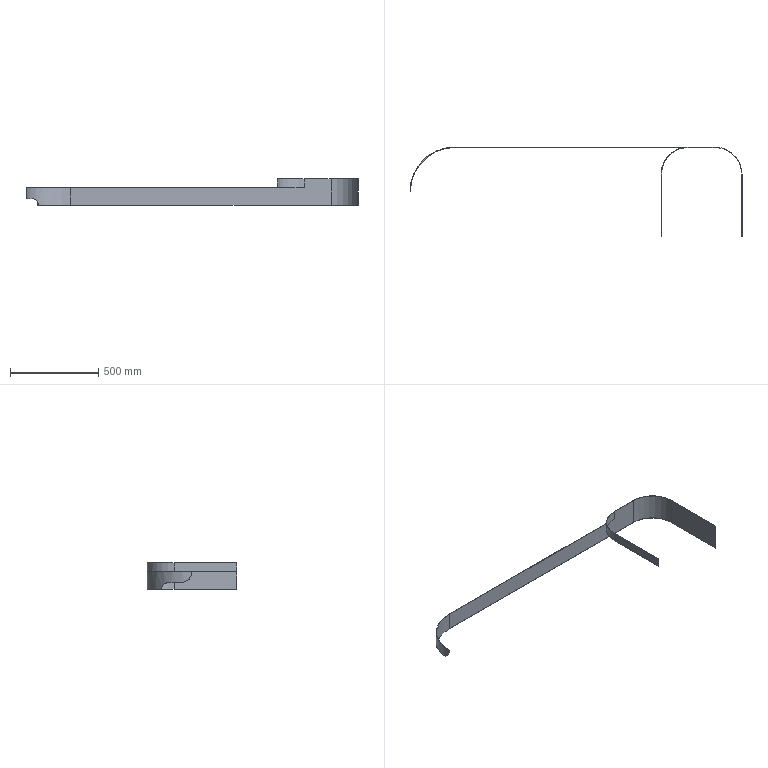Part | SolidWorks | features ICE 2, Extrusion 1 | 1 solid | 21 faces | box 1880 x 508 x 152.4 mm | volume 621350 mm3 | plane 13 | cylinder 8 | commonest cylinder face diameters 300.8 x2 304.8 x2 76.2 x1 127 x1 504 x1 508 x1
STEP:
#1=CARTESIAN_POINT('',(-215.391,134.62,-63.5));
#2=VERTEX_POINT('',#1);
#3=CARTESIAN_POINT('',(-186.236,172.72,-101.6));
#4=VERTEX_POINT('',#3);
#5=CARTESIAN_POINT('',(-215.391,134.62,-63.5));
#6=CARTESIAN_POINT('',(-213.888,137.025,-63.5));
#7=CARTESIAN_POINT('',(-212.368,139.368,-63.725));
#8=CARTESIAN_POINT('',(-209.293,143.945,-64.585));
#9=CARTESIAN_POINT('',(-207.739,146.177,-65.22));
#10=CARTESIAN_POINT('',(-205.78,148.9,-66.272));
#11=CARTESIAN_POINT('',(-205.387,149.441,-66.496));
#12=CARTESIAN_POINT('',(-204.6,150.517,-66.97));
#13=CARTESIAN_POINT('',(-204.206,151.05,-67.22));
#14=CARTESIAN_POINT('',(-203.034,152.627,-68.004));
#15=CARTESIAN_POINT('',(-202.26,153.651,-68.573));
#16=CARTESIAN_POINT('',(-199.965,156.64,-70.42));
#17=CARTESIAN_POINT('',(-198.471,158.526,-71.836));
#18=CARTESIAN_POINT('',(-196.304,161.19,-74.267));
#19=CARTESIAN_POINT('',(-195.593,162.051,-75.129));
#20=CARTESIAN_POINT('',(-194.206,163.711,-76.966));
#21=CARTESIAN_POINT('',(-193.538,164.499,-77.927));
#22=CARTESIAN_POINT('',(-192.262,165.989,-79.939));
#23=CARTESIAN_POINT('',(-191.654,166.69,-80.991));
#24=CARTESIAN_POINT('',(-190.504,168.003,-83.192));
#25=CARTESIAN_POINT('',(-189.963,168.613,-84.342));
#26=CARTESIAN_POINT('',(-189.213,169.454,-86.152));
#27=CARTESIAN_POINT('',(-188.974,169.72,-86.766));
#28=CARTESIAN_POINT('',(-188.524,170.219,-88.008));
#29=CARTESIAN_POINT('',(-188.313,170.454,-88.638));
#30=CARTESIAN_POINT('',(-187.719,171.108,-90.552));
#31=CARTESIAN_POINT('',(-187.378,171.481,-91.864));
#32=CARTESIAN_POINT('',(-186.959,171.938,-93.887));
#33=CARTESIAN_POINT('',(-186.834,172.073,-94.571));
#34=CARTESIAN_POINT('',(-186.618,172.307,-95.959));
#35=CARTESIAN_POINT('',(-186.528,172.405,-96.658));
#36=CARTESIAN_POINT('',(-186.31,172.64,-98.761));
#37=CARTESIAN_POINT('',(-186.236,172.72,-100.174));
#38=CARTESIAN_POINT('',(-186.236,172.72,-101.6));
#39=B_SPLINE_CURVE_WITH_KNOTS('',3,(#5,#6,#7,#8,#9,#10,#11,#12,#13,#14,#15,#16,#17,#18,#19,#20,#21,#22,#23,#24,#25,#26,#27,#28,#29,#30,#31,#32,#33,#34,#35,#36,#37,#38),.UNSPECIFIED.,.F.,.F.,(4,2,2,2,2,2,2,2,2,2,2,2,2,2,2,2,4),(0.,0.008368,0.01674,0.01883,0.02092,0.0251,0.03347,0.03765,0.04184,0.04602,0.05021,0.0523,0.05439,0.05857,0.06066,0.06276,0.06694),.UNSPECIFIED.);
#40=EDGE_CURVE('',#2,#4,#39,.T.);
#41=ORIENTED_EDGE('',*,*,#40,.F.);
#42=CARTESIAN_POINT('',(-245.934,63.5,-63.5));
#43=VERTEX_POINT('',#42);
#44=CARTESIAN_POINT('',(0.,0.,-63.5));
#45=DIRECTION('',(0.,0.,-1.));
#46=DIRECTION('',(1.,0.,0.));
#47=AXIS2_PLACEMENT_3D('',#44,#45,#46);
#48=CIRCLE('',#47,254.);
#49=EDGE_CURVE('',#43,#2,#48,.T.);
#50=ORIENTED_EDGE('',*,*,#49,.F.);
#51=CARTESIAN_POINT('',(-254.,0.,0.));
#52=VERTEX_POINT('',#51);
#53=CARTESIAN_POINT('',(-254.,0.,0.));
#54=CARTESIAN_POINT('',(-254.,0.,-4.22));
#55=CARTESIAN_POINT('',(-254.001,0.4165,-8.369));
#56=CARTESIAN_POINT('',(-253.995,1.64,-14.49));
#57=CARTESIAN_POINT('',(-253.992,2.149,-16.514));
#58=CARTESIAN_POINT('',(-253.982,3.066,-19.523));
#59=CARTESIAN_POINT('',(-253.978,3.399,-20.523));
#60=CARTESIAN_POINT('',(-253.967,4.113,-22.506));
#61=CARTESIAN_POINT('',(-253.961,4.493,-23.484));
#62=CARTESIAN_POINT('',(-253.922,6.507,-28.312));
#63=CARTESIAN_POINT('',(-253.869,8.479,-31.975));
#64=CARTESIAN_POINT('',(-253.745,11.391,-36.305));
#65=CARTESIAN_POINT('',(-253.717,11.996,-37.158));
#66=CARTESIAN_POINT('',(-253.655,13.252,-38.839));
#67=CARTESIAN_POINT('',(-253.62,13.905,-39.67));
#68=CARTESIAN_POINT('',(-253.504,15.916,-42.1));
#69=CARTESIAN_POINT('',(-253.413,17.326,-43.641));
#70=CARTESIAN_POINT('',(-253.084,21.757,-48.032));
#71=CARTESIAN_POINT('',(-252.793,24.978,-50.654));
#72=CARTESIAN_POINT('',(-252.301,29.343,-53.541));
#73=CARTESIAN_POINT('',(-252.196,30.235,-54.099));
#74=CARTESIAN_POINT('',(-251.974,32.032,-55.165));
#75=CARTESIAN_POINT('',(-251.857,32.941,-55.673));
#76=CARTESIAN_POINT('',(-251.487,35.693,-57.125));
#77=CARTESIAN_POINT('',(-251.215,37.563,-57.998));
#78=CARTESIAN_POINT('',(-250.615,41.374,-59.556));
#79=CARTESIAN_POINT('',(-250.288,43.314,-60.242));
#80=CARTESIAN_POINT('',(-249.751,46.277,-61.128));
#81=CARTESIAN_POINT('',(-249.564,47.273,-61.4));
#82=CARTESIAN_POINT('',(-249.175,49.283,-61.897));
#83=CARTESIAN_POINT('',(-248.973,50.294,-62.12));
#84=CARTESIAN_POINT('',(-247.931,55.349,-63.109));
#85=CARTESIAN_POINT('',(-246.989,59.415,-63.5));
#86=CARTESIAN_POINT('',(-245.934,63.5,-63.5));
#87=B_SPLINE_CURVE_WITH_KNOTS('',3,(#53,#54,#55,#56,#57,#58,#59,#60,#61,#62,#63,#64,#65,#66,#67,#68,#69,#70,#71,#72,#73,#74,#75,#76,#77,#78,#79,#80,#81,#82,#83,#84,#85,#86),.UNSPECIFIED.,.F.,.F.,(4,2,2,2,2,2,2,2,2,2,2,2,2,2,2,2,4),(0.,0.01248,0.01872,0.02184,0.02496,0.03744,0.04056,0.04368,0.04992,0.0624,0.06552,0.06864,0.07488,0.08112,0.08424,0.08736,0.09984),.UNSPECIFIED.);
#88=EDGE_CURVE('',#52,#43,#87,.T.);
#89=ORIENTED_EDGE('',*,*,#88,.F.);
#90=CARTESIAN_POINT('',(0.,254.,0.));
#91=VERTEX_POINT('',#90);
#92=CARTESIAN_POINT('',(0.,0.,0.));
#93=DIRECTION('',(0.,0.,1.));
#94=DIRECTION('',(1.,0.,0.));
#95=AXIS2_PLACEMENT_3D('',#92,#93,#94);
#96=CIRCLE('',#95,254.);
#97=EDGE_CURVE('',#91,#52,#96,.T.);
#98=ORIENTED_EDGE('',*,*,#97,.F.);
#99=CARTESIAN_POINT('',(0.,254.,-101.6));
#100=VERTEX_POINT('',#99);
#101=CARTESIAN_POINT('',(0.,254.,-101.6));
#102=DIRECTION('',(0.,0.,1.));
#103=VECTOR('',#102,1000.);
#104=LINE('',#101,#103);
#105=EDGE_CURVE('',#100,#91,#104,.T.);
#106=ORIENTED_EDGE('',*,*,#105,.F.);
#107=CARTESIAN_POINT('',(0.,0.,-101.6));
#108=DIRECTION('',(0.,0.,1.));
#109=DIRECTION('',(1.,0.,0.));
#110=AXIS2_PLACEMENT_3D('',#107,#108,#109);
#111=CIRCLE('',#110,254.);
#112=EDGE_CURVE('',#100,#4,#111,.T.);
#113=ORIENTED_EDGE('',*,*,#112,.T.);
#114=EDGE_LOOP('',(#41,#50,#89,#98,#106,#113));
#115=FACE_OUTER_BOUND('',#114,.T.);
#116=CARTESIAN_POINT('',(0.,0.,-101.6));
#117=DIRECTION('',(0.,0.,1.));
#118=DIRECTION('',(1.,0.,0.));
#119=AXIS2_PLACEMENT_3D('',#116,#117,#118);
#120=CYLINDRICAL_SURFACE('',#119,254.);
#121=ADVANCED_FACE('',(#115),#120,.T.);
#122=CARTESIAN_POINT('',(1320.8,254.,0.));
#123=VERTEX_POINT('',#122);
#124=CARTESIAN_POINT('',(0.,254.,0.));
#125=DIRECTION('',(-1.,0.,0.));
#126=VECTOR('',#125,1000.);
#127=LINE('',#124,#126);
#128=EDGE_CURVE('',#123,#91,#127,.T.);
#129=ORIENTED_EDGE('',*,*,#128,.F.);
#130=CARTESIAN_POINT('',(1320.8,254.,50.8));
#131=VERTEX_POINT('',#130);
#132=CARTESIAN_POINT('',(1320.8,254.,50.8));
#133=DIRECTION('',(0.,0.,-1.));
#134=VECTOR('',#133,1000.);
#135=LINE('',#132,#134);
#136=EDGE_CURVE('',#131,#123,#135,.T.);
#137=ORIENTED_EDGE('',*,*,#136,.F.);
#138=CARTESIAN_POINT('',(1473.2,254.,50.8));
#139=VERTEX_POINT('',#138);
#140=CARTESIAN_POINT('',(1473.2,254.,50.8));
#141=DIRECTION('',(-1.,0.,0.));
#142=VECTOR('',#141,1000.);
#143=LINE('',#140,#142);
#144=EDGE_CURVE('',#139,#131,#143,.T.);
#145=ORIENTED_EDGE('',*,*,#144,.F.);
#146=CARTESIAN_POINT('',(1473.2,254.,-101.6));
#147=VERTEX_POINT('',#146);
#148=CARTESIAN_POINT('',(1473.2,254.,-101.6));
#149=DIRECTION('',(0.,0.,1.));
#150=VECTOR('',#149,1000.);
#151=LINE('',#148,#150);
#152=EDGE_CURVE('',#147,#139,#151,.T.);
#153=ORIENTED_EDGE('',*,*,#152,.F.);
#154=CARTESIAN_POINT('',(0.,254.,-101.6));
#155=DIRECTION('',(-1.,0.,0.));
#156=VECTOR('',#155,1000.);
#157=LINE('',#154,#156);
#158=EDGE_CURVE('',#147,#100,#157,.T.);
#159=ORIENTED_EDGE('',*,*,#158,.T.);
#160=ORIENTED_EDGE('',*,*,#105,.T.);
#161=EDGE_LOOP('',(#129,#137,#145,#153,#159,#160));
#162=FACE_OUTER_BOUND('',#161,.T.);
#163=CARTESIAN_POINT('',(0.,254.,-101.6));
#164=DIRECTION('',(0.,1.,0.));
#165=DIRECTION('',(0.,0.,1.));
#166=AXIS2_PLACEMENT_3D('',#163,#164,#165);
#167=PLANE('',#166);
#168=ADVANCED_FACE('',(#162),#167,.T.);
#169=ORIENTED_EDGE('',*,*,#152,.T.);
#170=CARTESIAN_POINT('',(1625.6,101.6,50.8));
#171=VERTEX_POINT('',#170);
#172=CARTESIAN_POINT('',(1473.2,101.6,50.8));
#173=DIRECTION('',(0.,0.,1.));
#174=DIRECTION('',(1.,0.,0.));
#175=AXIS2_PLACEMENT_3D('',#172,#173,#174);
#176=CIRCLE('',#175,152.4);
#177=EDGE_CURVE('',#171,#139,#176,.T.);
#178=ORIENTED_EDGE('',*,*,#177,.F.);
#179=CARTESIAN_POINT('',(1625.6,101.6,-101.6));
#180=VERTEX_POINT('',#179);
#181=CARTESIAN_POINT('',(1625.6,101.6,-101.6));
#182=DIRECTION('',(0.,0.,1.));
#183=VECTOR('',#182,1000.);
#184=LINE('',#181,#183);
#185=EDGE_CURVE('',#180,#171,#184,.T.);
#186=ORIENTED_EDGE('',*,*,#185,.F.);
#187=CARTESIAN_POINT('',(1473.2,101.6,-101.6));
#188=DIRECTION('',(0.,0.,1.));
#189=DIRECTION('',(-1.,0.,0.));
#190=AXIS2_PLACEMENT_3D('',#187,#188,#189);
#191=CIRCLE('',#190,152.4);
#192=EDGE_CURVE('',#180,#147,#191,.T.);
#193=ORIENTED_EDGE('',*,*,#192,.T.);
#194=EDGE_LOOP('',(#169,#178,#186,#193));
#195=FACE_OUTER_BOUND('',#194,.T.);
#196=CARTESIAN_POINT('',(1473.2,101.6,-101.6));
#197=DIRECTION('',(0.,0.,1.));
#198=DIRECTION('',(1.,0.,0.));
#199=AXIS2_PLACEMENT_3D('',#196,#197,#198);
#200=CYLINDRICAL_SURFACE('',#199,152.4);
#201=ADVANCED_FACE('',(#195),#200,.T.);
#202=ORIENTED_EDGE('',*,*,#185,.T.);
#203=CARTESIAN_POINT('',(1625.6,-254.,50.8));
#204=VERTEX_POINT('',#203);
#205=CARTESIAN_POINT('',(1625.6,-254.,50.8));
#206=DIRECTION('',(0.,1.,0.));
#207=VECTOR('',#206,1000.);
#208=LINE('',#205,#207);
#209=EDGE_CURVE('',#204,#171,#208,.T.);
#210=ORIENTED_EDGE('',*,*,#209,.F.);
#211=CARTESIAN_POINT('',(1625.6,-254.,-101.6));
#212=VERTEX_POINT('',#211);
#213=CARTESIAN_POINT('',(1625.6,-254.,-101.6));
#214=DIRECTION('',(0.,0.,1.));
#215=VECTOR('',#214,1000.);
#216=LINE('',#213,#215);
#217=EDGE_CURVE('',#212,#204,#216,.T.);
#218=ORIENTED_EDGE('',*,*,#217,.F.);
#219=CARTESIAN_POINT('',(1625.6,101.6,-101.6));
#220=DIRECTION('',(0.,1.,0.));
#221=VECTOR('',#220,1000.);
#222=LINE('',#219,#221);
#223=EDGE_CURVE('',#212,#180,#222,.T.);
#224=ORIENTED_EDGE('',*,*,#223,.T.);
#225=EDGE_LOOP('',(#202,#210,#218,#224));
#226=FACE_OUTER_BOUND('',#225,.T.);
#227=CARTESIAN_POINT('',(1625.6,101.6,-101.6));
#228=DIRECTION('',(1.,0.,0.));
#229=DIRECTION('',(0.,0.,-1.));
#230=AXIS2_PLACEMENT_3D('',#227,#228,#229);
#231=PLANE('',#230);
#232=ADVANCED_FACE('',(#226),#231,.T.);
#233=ORIENTED_EDGE('',*,*,#217,.T.);
#234=CARTESIAN_POINT('',(1623.6,-254.,50.8));
#235=VERTEX_POINT('',#234);
#236=CARTESIAN_POINT('',(1623.6,-254.,50.8));
#237=DIRECTION('',(1.,0.,0.));
#238=VECTOR('',#237,1000.);
#239=LINE('',#236,#238);
#240=EDGE_CURVE('',#235,#204,#239,.T.);
#241=ORIENTED_EDGE('',*,*,#240,.F.);
#242=CARTESIAN_POINT('',(1623.6,-254.,-101.6));
#243=VERTEX_POINT('',#242);
#244=CARTESIAN_POINT('',(1623.6,-254.,-101.6));
#245=DIRECTION('',(0.,0.,1.));
#246=VECTOR('',#245,1000.);
#247=LINE('',#244,#246);
#248=EDGE_CURVE('',#243,#235,#247,.T.);
#249=ORIENTED_EDGE('',*,*,#248,.F.);
#250=CARTESIAN_POINT('',(1623.6,-254.,-101.6));
#251=DIRECTION('',(1.,0.,0.));
#252=VECTOR('',#251,1000.);
#253=LINE('',#250,#252);
#254=EDGE_CURVE('',#243,#212,#253,.T.);
#255=ORIENTED_EDGE('',*,*,#254,.T.);
#256=EDGE_LOOP('',(#233,#241,#249,#255));
#257=FACE_OUTER_BOUND('',#256,.T.);
#258=CARTESIAN_POINT('',(1623.6,-254.,-101.6));
#259=DIRECTION('',(0.,-1.,0.));
#260=DIRECTION('',(0.,0.,-1.));
#261=AXIS2_PLACEMENT_3D('',#258,#259,#260);
#262=PLANE('',#261);
#263=ADVANCED_FACE('',(#257),#262,.T.);
#264=ORIENTED_EDGE('',*,*,#248,.T.);
#265=CARTESIAN_POINT('',(1623.6,101.6,50.8));
#266=VERTEX_POINT('',#265);
#267=CARTESIAN_POINT('',(1623.6,-254.,50.8));
#268=DIRECTION('',(0.,-1.,0.));
#269=VECTOR('',#268,1000.);
#270=LINE('',#267,#269);
#271=EDGE_CURVE('',#266,#235,#270,.T.);
#272=ORIENTED_EDGE('',*,*,#271,.F.);
#273=CARTESIAN_POINT('',(1623.6,101.6,-101.6));
#274=VERTEX_POINT('',#273);
#275=CARTESIAN_POINT('',(1623.6,101.6,-101.6));
#276=DIRECTION('',(0.,0.,1.));
#277=VECTOR('',#276,1000.);
#278=LINE('',#275,#277);
#279=EDGE_CURVE('',#274,#266,#278,.T.);
#280=ORIENTED_EDGE('',*,*,#279,.F.);
#281=CARTESIAN_POINT('',(1623.6,101.6,-101.6));
#282=DIRECTION('',(0.,-1.,0.));
#283=VECTOR('',#282,1000.);
#284=LINE('',#281,#283);
#285=EDGE_CURVE('',#274,#243,#284,.T.);
#286=ORIENTED_EDGE('',*,*,#285,.T.);
#287=EDGE_LOOP('',(#264,#272,#280,#286));
#288=FACE_OUTER_BOUND('',#287,.T.);
#289=CARTESIAN_POINT('',(1623.6,101.6,-101.6));
#290=DIRECTION('',(-1.,0.,0.));
#291=DIRECTION('',(0.,0.,1.));
#292=AXIS2_PLACEMENT_3D('',#289,#290,#291);
#293=PLANE('',#292);
#294=ADVANCED_FACE('',(#288),#293,.T.);
#295=ORIENTED_EDGE('',*,*,#279,.T.);
#296=CARTESIAN_POINT('',(1473.2,252.,50.8));
#297=VERTEX_POINT('',#296);
#298=CARTESIAN_POINT('',(1473.2,101.6,50.8));
#299=DIRECTION('',(0.,0.,-1.));
#300=DIRECTION('',(1.,0.,0.));
#301=AXIS2_PLACEMENT_3D('',#298,#299,#300);
#302=CIRCLE('',#301,150.4);
#303=EDGE_CURVE('',#297,#266,#302,.T.);
#304=ORIENTED_EDGE('',*,*,#303,.F.);
#305=CARTESIAN_POINT('',(1473.2,252.,-101.6));
#306=VERTEX_POINT('',#305);
#307=CARTESIAN_POINT('',(1473.2,252.,-101.6));
#308=DIRECTION('',(0.,0.,1.));
#309=VECTOR('',#308,1000.);
#310=LINE('',#307,#309);
#311=EDGE_CURVE('',#306,#297,#310,.T.);
#312=ORIENTED_EDGE('',*,*,#311,.F.);
#313=CARTESIAN_POINT('',(1473.2,101.6,-101.6));
#314=DIRECTION('',(0.,0.,-1.));
#315=DIRECTION('',(-1.,0.,0.));
#316=AXIS2_PLACEMENT_3D('',#313,#314,#315);
#317=CIRCLE('',#316,150.4);
#318=EDGE_CURVE('',#306,#274,#317,.T.);
#319=ORIENTED_EDGE('',*,*,#318,.T.);
#320=EDGE_LOOP('',(#295,#304,#312,#319));
#321=FACE_OUTER_BOUND('',#320,.T.);
#322=CARTESIAN_POINT('',(1473.2,101.6,-101.6));
#323=DIRECTION('',(0.,0.,1.));
#324=DIRECTION('',(1.,0.,0.));
#325=AXIS2_PLACEMENT_3D('',#322,#323,#324);
#326=CYLINDRICAL_SURFACE('',#325,150.4);
#327=ADVANCED_FACE('',(#321),#326,.F.);
#328=CARTESIAN_POINT('',(0.,252.,0.));
#329=VERTEX_POINT('',#328);
#330=CARTESIAN_POINT('',(1296.191,252.,0.));
#331=VERTEX_POINT('',#330);
#332=CARTESIAN_POINT('',(0.,252.,0.));
#333=DIRECTION('',(1.,0.,0.));
#334=VECTOR('',#333,1000.);
#335=LINE('',#332,#334);
#336=EDGE_CURVE('',#329,#331,#335,.T.);
#337=ORIENTED_EDGE('',*,*,#336,.F.);
#338=CARTESIAN_POINT('',(0.,252.,-101.6));
#339=VERTEX_POINT('',#338);
#340=CARTESIAN_POINT('',(0.,252.,-101.6));
#341=DIRECTION('',(0.,0.,1.));
#342=VECTOR('',#341,1000.);
#343=LINE('',#340,#342);
#344=EDGE_CURVE('',#339,#329,#343,.T.);
#345=ORIENTED_EDGE('',*,*,#344,.F.);
#346=CARTESIAN_POINT('',(0.,252.,-101.6));
#347=DIRECTION('',(1.,0.,0.));
#348=VECTOR('',#347,1000.);
#349=LINE('',#346,#348);
#350=EDGE_CURVE('',#339,#306,#349,.T.);
#351=ORIENTED_EDGE('',*,*,#350,.T.);
#352=ORIENTED_EDGE('',*,*,#311,.T.);
#353=CARTESIAN_POINT('',(1320.8,252.,50.8));
#354=VERTEX_POINT('',#353);
#355=CARTESIAN_POINT('',(1473.2,252.,50.8));
#356=DIRECTION('',(1.,0.,0.));
#357=VECTOR('',#356,1000.);
#358=LINE('',#355,#357);
#359=EDGE_CURVE('',#354,#297,#358,.T.);
#360=ORIENTED_EDGE('',*,*,#359,.F.);
#361=CARTESIAN_POINT('',(1320.8,252.,0.));
#362=VERTEX_POINT('',#361);
#363=CARTESIAN_POINT('',(1320.8,252.,50.8));
#364=DIRECTION('',(0.,0.,-1.));
#365=VECTOR('',#364,1000.);
#366=LINE('',#363,#365);
#367=EDGE_CURVE('',#354,#362,#366,.T.);
#368=ORIENTED_EDGE('',*,*,#367,.T.);
#369=CARTESIAN_POINT('',(0.,252.,0.));
#370=DIRECTION('',(1.,0.,0.));
#371=VECTOR('',#370,1000.);
#372=LINE('',#369,#371);
#373=EDGE_CURVE('',#331,#362,#372,.T.);
#374=ORIENTED_EDGE('',*,*,#373,.F.);
#375=EDGE_LOOP('',(#337,#345,#351,#352,#360,#368,#374));
#376=FACE_OUTER_BOUND('',#375,.T.);
#377=CARTESIAN_POINT('',(0.,252.,-101.6));
#378=DIRECTION('',(0.,-1.,0.));
#379=DIRECTION('',(0.,0.,-1.));
#380=AXIS2_PLACEMENT_3D('',#377,#378,#379);
#381=PLANE('',#380);
#382=ADVANCED_FACE('',(#376),#381,.T.);
#383=CARTESIAN_POINT('',(-183.499,172.72,-101.6));
#384=VERTEX_POINT('',#383);
#385=CARTESIAN_POINT('',(-213.029,134.62,-63.5));
#386=VERTEX_POINT('',#385);
#387=CARTESIAN_POINT('',(-183.499,172.72,-101.6));
#388=CARTESIAN_POINT('',(-183.499,172.72,-98.744));
#389=CARTESIAN_POINT('',(-183.798,172.403,-95.969));
#390=CARTESIAN_POINT('',(-184.503,171.647,-92.594));
#391=CARTESIAN_POINT('',(-184.661,171.477,-91.923));
#392=CARTESIAN_POINT('',(-185.009,171.102,-90.592));
#393=CARTESIAN_POINT('',(-185.197,170.898,-89.939));
#394=CARTESIAN_POINT('',(-185.802,170.241,-88.014));
#395=CARTESIAN_POINT('',(-186.257,169.743,-86.777));
#396=CARTESIAN_POINT('',(-187.261,168.635,-84.387));
#397=CARTESIAN_POINT('',(-187.809,168.025,-83.232));
#398=CARTESIAN_POINT('',(-188.986,166.7,-81.005));
#399=CARTESIAN_POINT('',(-189.606,165.996,-79.95));
#400=CARTESIAN_POINT('',(-191.541,163.768,-76.937));
#401=CARTESIAN_POINT('',(-192.933,162.13,-75.131));
#402=CARTESIAN_POINT('',(-195.135,159.46,-72.686));
#403=CARTESIAN_POINT('',(-195.891,158.531,-71.914));
#404=CARTESIAN_POINT('',(-197.413,156.632,-70.479));
#405=CARTESIAN_POINT('',(-198.183,155.658,-69.813));
#406=CARTESIAN_POINT('',(-200.509,152.664,-67.962));
#407=CARTESIAN_POINT('',(-202.086,150.574,-66.922));
#408=CARTESIAN_POINT('',(-204.478,147.291,-65.65));
#409=CARTESIAN_POINT('',(-205.272,146.182,-65.278));
#410=CARTESIAN_POINT('',(-206.85,143.94,-64.639));
#411=CARTESIAN_POINT('',(-207.635,142.807,-64.372));
#412=CARTESIAN_POINT('',(-209.973,139.366,-63.725));
#413=CARTESIAN_POINT('',(-211.512,137.021,-63.5));
#414=CARTESIAN_POINT('',(-213.029,134.62,-63.5));
#415=B_SPLINE_CURVE_WITH_KNOTS('',3,(#387,#388,#389,#390,#391,#392,#393,#394,#395,#396,#397,#398,#399,#400,#401,#402,#403,#404,#405,#406,#407,#408,#409,#410,#411,#412,#413,#414),.UNSPECIFIED.,.F.,.F.,(4,2,2,2,2,2,2,2,2,2,2,2,2,4),(0.,0.008421,0.01053,0.01263,0.01684,0.02105,0.02526,0.03368,0.03789,0.0421,0.05052,0.05473,0.05894,0.06737),.UNSPECIFIED.);
#416=EDGE_CURVE('',#384,#386,#415,.T.);
#417=ORIENTED_EDGE('',*,*,#416,.F.);
#418=CARTESIAN_POINT('',(0.,0.,-101.6));
#419=DIRECTION('',(0.,0.,-1.));
#420=DIRECTION('',(1.,0.,0.));
#421=AXIS2_PLACEMENT_3D('',#418,#419,#420);
#422=CIRCLE('',#421,252.);
#423=EDGE_CURVE('',#384,#339,#422,.T.);
#424=ORIENTED_EDGE('',*,*,#423,.T.);
#425=ORIENTED_EDGE('',*,*,#344,.T.);
#426=CARTESIAN_POINT('',(-252.,0.,0.));
#427=VERTEX_POINT('',#426);
#428=CARTESIAN_POINT('',(0.,0.,0.));
#429=DIRECTION('',(0.,0.,-1.));
#430=DIRECTION('',(1.,0.,0.));
#431=AXIS2_PLACEMENT_3D('',#428,#429,#430);
#432=CIRCLE('',#431,252.);
#433=EDGE_CURVE('',#427,#329,#432,.T.);
#434=ORIENTED_EDGE('',*,*,#433,.F.);
#435=CARTESIAN_POINT('',(-243.868,63.5,-63.5));
#436=VERTEX_POINT('',#435);
#437=CARTESIAN_POINT('',(-243.868,63.5,-63.5));
#438=CARTESIAN_POINT('',(-244.931,59.417,-63.5));
#439=CARTESIAN_POINT('',(-245.875,55.373,-63.11));
#440=CARTESIAN_POINT('',(-247.125,49.369,-61.941));
#441=CARTESIAN_POINT('',(-247.515,47.377,-61.454));
#442=CARTESIAN_POINT('',(-248.059,44.407,-60.57));
#443=CARTESIAN_POINT('',(-248.234,43.417,-60.25));
#444=CARTESIAN_POINT('',(-248.569,41.455,-59.56));
#445=CARTESIAN_POINT('',(-248.729,40.485,-59.192));
#446=CARTESIAN_POINT('',(-249.49,35.693,-57.238));
#447=CARTESIAN_POINT('',(-249.98,32.038,-55.314));
#448=CARTESIAN_POINT('',(-250.475,27.699,-52.456));
#449=CARTESIAN_POINT('',(-250.568,26.843,-51.861));
#450=CARTESIAN_POINT('',(-250.743,25.154,-50.625));
#451=CARTESIAN_POINT('',(-250.825,24.319,-49.982));
#452=CARTESIAN_POINT('',(-251.054,21.874,-47.999));
#453=CARTESIAN_POINT('',(-251.184,20.321,-46.606));
#454=CARTESIAN_POINT('',(-251.516,15.884,-42.217));
#455=CARTESIAN_POINT('',(-251.664,13.222,-39.014));
#456=CARTESIAN_POINT('',(-251.791,10.28,-34.655));
#457=CARTESIAN_POINT('',(-251.813,9.711,-33.765));
#458=CARTESIAN_POINT('',(-251.853,8.624,-31.969));
#459=CARTESIAN_POINT('',(-251.87,8.105,-31.06));
#460=CARTESIAN_POINT('',(-251.915,6.618,-28.303));
#461=CARTESIAN_POINT('',(-251.936,5.722,-26.424));
#462=CARTESIAN_POINT('',(-251.968,4.116,-22.585));
#463=CARTESIAN_POINT('',(-251.978,3.406,-20.624));
#464=CARTESIAN_POINT('',(-251.988,2.485,-17.622));
#465=CARTESIAN_POINT('',(-251.991,2.202,-16.61));
#466=CARTESIAN_POINT('',(-251.995,1.684,-14.566));
#467=CARTESIAN_POINT('',(-251.996,1.451,-13.539));
#468=CARTESIAN_POINT('',(-252.001,0.4166,-8.39));
#469=CARTESIAN_POINT('',(-252.,0.,-4.22));
#470=CARTESIAN_POINT('',(-252.,0.,0.));
#471=B_SPLINE_CURVE_WITH_KNOTS('',3,(#437,#438,#439,#440,#441,#442,#443,#444,#445,#446,#447,#448,#449,#450,#451,#452,#453,#454,#455,#456,#457,#458,#459,#460,#461,#462,#463,#464,#465,#466,#467,#468,#469,#470),.UNSPECIFIED.,.F.,.F.,(4,2,2,2,2,2,2,2,2,2,2,2,2,2,2,2,4),(0.,0.01248,0.01872,0.02184,0.02497,0.03745,0.04057,0.04369,0.04993,0.06241,0.06553,0.06865,0.0749,0.08114,0.08426,0.08738,0.09986),.UNSPECIFIED.);
#472=EDGE_CURVE('',#436,#427,#471,.T.);
#473=ORIENTED_EDGE('',*,*,#472,.F.);
#474=CARTESIAN_POINT('',(0.,0.,-63.5));
#475=DIRECTION('',(0.,0.,1.));
#476=DIRECTION('',(1.,0.,0.));
#477=AXIS2_PLACEMENT_3D('',#474,#475,#476);
#478=CIRCLE('',#477,252.);
#479=EDGE_CURVE('',#386,#436,#478,.T.);
#480=ORIENTED_EDGE('',*,*,#479,.F.);
#481=EDGE_LOOP('',(#417,#424,#425,#434,#473,#480));
#482=FACE_OUTER_BOUND('',#481,.T.);
#483=CARTESIAN_POINT('',(0.,0.,-101.6));
#484=DIRECTION('',(0.,0.,1.));
#485=DIRECTION('',(1.,0.,0.));
#486=AXIS2_PLACEMENT_3D('',#483,#484,#485);
#487=CYLINDRICAL_SURFACE('',#486,252.);
#488=ADVANCED_FACE('',(#482),#487,.F.);
#489=ORIENTED_EDGE('',*,*,#423,.F.);
#490=CARTESIAN_POINT('',(-800.,172.72,-101.6));
#491=DIRECTION('',(-1.,0.,0.));
#492=VECTOR('',#491,1000.);
#493=LINE('',#490,#492);
#494=EDGE_CURVE('',#384,#4,#493,.T.);
#495=ORIENTED_EDGE('',*,*,#494,.T.);
#496=ORIENTED_EDGE('',*,*,#112,.F.);
#497=ORIENTED_EDGE('',*,*,#158,.F.);
#498=ORIENTED_EDGE('',*,*,#192,.F.);
#499=ORIENTED_EDGE('',*,*,#223,.F.);
#500=ORIENTED_EDGE('',*,*,#254,.F.);
#501=ORIENTED_EDGE('',*,*,#285,.F.);
#502=ORIENTED_EDGE('',*,*,#318,.F.);
#503=ORIENTED_EDGE('',*,*,#350,.F.);
#504=EDGE_LOOP('',(#489,#495,#496,#497,#498,#499,#500,#501,#502,#503));
#505=FACE_OUTER_BOUND('',#504,.T.);
#506=CARTESIAN_POINT('',(0.,0.,-101.6));
#507=DIRECTION('',(0.,0.,1.));
#508=DIRECTION('',(1.,0.,0.));
#509=AXIS2_PLACEMENT_3D('',#506,#507,#508);
#510=PLANE('',#509);
#511=ADVANCED_FACE('',(#505),#510,.F.);
#512=CARTESIAN_POINT('',(1320.8,101.6,0.));
#513=DIRECTION('',(0.,0.,1.));
#514=DIRECTION('',(-1.,0.,0.));
#515=AXIS2_PLACEMENT_3D('',#512,#513,#514);
#516=CIRCLE('',#515,152.4);
#517=EDGE_CURVE('',#123,#331,#516,.T.);
#518=ORIENTED_EDGE('',*,*,#517,.F.);
#519=ORIENTED_EDGE('',*,*,#128,.T.);
#520=ORIENTED_EDGE('',*,*,#97,.T.);
#521=CARTESIAN_POINT('',(-254.,0.,0.));
#522=DIRECTION('',(1.,0.,0.));
#523=VECTOR('',#522,1000.);
#524=LINE('',#521,#523);
#525=EDGE_CURVE('',#52,#427,#524,.T.);
#526=ORIENTED_EDGE('',*,*,#525,.T.);
#527=ORIENTED_EDGE('',*,*,#433,.T.);
#528=ORIENTED_EDGE('',*,*,#336,.T.);
#529=EDGE_LOOP('',(#518,#519,#520,#526,#527,#528));
#530=FACE_OUTER_BOUND('',#529,.T.);
#531=CARTESIAN_POINT('',(0.,0.,0.));
#532=DIRECTION('',(0.,0.,1.));
#533=DIRECTION('',(1.,0.,0.));
#534=AXIS2_PLACEMENT_3D('',#531,#532,#533);
#535=PLANE('',#534);
#536=ADVANCED_FACE('',(#530),#535,.T.);
#537=CARTESIAN_POINT('',(1168.4,101.6,0.));
#538=VERTEX_POINT('',#537);
#539=CARTESIAN_POINT('',(1320.8,101.6,0.));
#540=DIRECTION('',(0.,0.,1.));
#541=DIRECTION('',(-1.,0.,0.));
#542=AXIS2_PLACEMENT_3D('',#539,#540,#541);
#543=CIRCLE('',#542,152.4);
#544=EDGE_CURVE('',#331,#538,#543,.T.);
#545=ORIENTED_EDGE('',*,*,#544,.F.);
#546=ORIENTED_EDGE('',*,*,#373,.T.);
#547=CARTESIAN_POINT('',(1170.4,101.6,0.));
#548=VERTEX_POINT('',#547);
#549=CARTESIAN_POINT('',(1320.8,101.6,0.));
#550=DIRECTION('',(0.,0.,-1.));
#551=DIRECTION('',(-1.,0.,0.));
#552=AXIS2_PLACEMENT_3D('',#549,#550,#551);
#553=CIRCLE('',#552,150.4);
#554=EDGE_CURVE('',#548,#362,#553,.T.);
#555=ORIENTED_EDGE('',*,*,#554,.F.);
#556=CARTESIAN_POINT('',(1170.4,-254.,0.));
#557=VERTEX_POINT('',#556);
#558=CARTESIAN_POINT('',(1170.4,101.6,0.));
#559=DIRECTION('',(0.,1.,0.));
#560=VECTOR('',#559,1000.);
#561=LINE('',#558,#560);
#562=EDGE_CURVE('',#557,#548,#561,.T.);
#563=ORIENTED_EDGE('',*,*,#562,.F.);
#564=CARTESIAN_POINT('',(1168.4,-254.,0.));
#565=VERTEX_POINT('',#564);
#566=CARTESIAN_POINT('',(1168.4,-254.,0.));
#567=DIRECTION('',(1.,0.,0.));
#568=VECTOR('',#567,1000.);
#569=LINE('',#566,#568);
#570=EDGE_CURVE('',#565,#557,#569,.T.);
#571=ORIENTED_EDGE('',*,*,#570,.F.);
#572=CARTESIAN_POINT('',(1168.4,101.6,0.));
#573=DIRECTION('',(0.,-1.,0.));
#574=VECTOR('',#573,1000.);
#575=LINE('',#572,#574);
#576=EDGE_CURVE('',#538,#565,#575,.T.);
#577=ORIENTED_EDGE('',*,*,#576,.F.);
#578=EDGE_LOOP('',(#545,#546,#555,#563,#571,#577));
#579=FACE_OUTER_BOUND('',#578,.T.);
#580=CARTESIAN_POINT('',(1473.2,101.6,0.));
#581=DIRECTION('',(0.,0.,1.));
#582=DIRECTION('',(1.,0.,0.));
#583=AXIS2_PLACEMENT_3D('',#580,#581,#582);
#584=PLANE('',#583);
#585=ADVANCED_FACE('',(#579),#584,.F.);
#586=ORIENTED_EDGE('',*,*,#517,.T.);
#587=ORIENTED_EDGE('',*,*,#544,.T.);
#588=CARTESIAN_POINT('',(1168.4,101.6,50.8));
#589=VERTEX_POINT('',#588);
#590=CARTESIAN_POINT('',(1168.4,101.6,50.8));
#591=DIRECTION('',(0.,0.,-1.));
#592=VECTOR('',#591,1000.);
#593=LINE('',#590,#592);
#594=EDGE_CURVE('',#589,#538,#593,.T.);
#595=ORIENTED_EDGE('',*,*,#594,.F.);
#596=CARTESIAN_POINT('',(1320.8,101.6,50.8));
#597=DIRECTION('',(0.,0.,1.));
#598=DIRECTION('',(-1.,0.,0.));
#599=AXIS2_PLACEMENT_3D('',#596,#597,#598);
#600=CIRCLE('',#599,152.4);
#601=EDGE_CURVE('',#131,#589,#600,.T.);
#602=ORIENTED_EDGE('',*,*,#601,.F.);
#603=ORIENTED_EDGE('',*,*,#136,.T.);
#604=EDGE_LOOP('',(#586,#587,#595,#602,#603));
#605=FACE_OUTER_BOUND('',#604,.T.);
#606=CARTESIAN_POINT('',(1320.8,101.6,50.8));
#607=DIRECTION('',(0.,0.,-1.));
#608=DIRECTION('',(-1.,0.,0.));
#609=AXIS2_PLACEMENT_3D('',#606,#607,#608);
#610=CYLINDRICAL_SURFACE('',#609,152.4);
#611=ADVANCED_FACE('',(#605),#610,.T.);
#612=ORIENTED_EDGE('',*,*,#576,.T.);
#613=CARTESIAN_POINT('',(1168.4,-254.,50.8));
#614=VERTEX_POINT('',#613);
#615=CARTESIAN_POINT('',(1168.4,-254.,50.8));
#616=DIRECTION('',(0.,0.,-1.));
#617=VECTOR('',#616,1000.);
#618=LINE('',#615,#617);
#619=EDGE_CURVE('',#614,#565,#618,.T.);
#620=ORIENTED_EDGE('',*,*,#619,.F.);
#621=CARTESIAN_POINT('',(1168.4,101.6,50.8));
#622=DIRECTION('',(0.,-1.,0.));
#623=VECTOR('',#622,1000.);
#624=LINE('',#621,#623);
#625=EDGE_CURVE('',#589,#614,#624,.T.);
#626=ORIENTED_EDGE('',*,*,#625,.F.);
#627=ORIENTED_EDGE('',*,*,#594,.T.);
#628=EDGE_LOOP('',(#612,#620,#626,#627));
#629=FACE_OUTER_BOUND('',#628,.T.);
#630=CARTESIAN_POINT('',(1168.4,101.6,50.8));
#631=DIRECTION('',(1.,0.,0.));
#632=DIRECTION('',(0.,1.,0.));
#633=AXIS2_PLACEMENT_3D('',#630,#631,#632);
#634=PLANE('',#633);
#635=ADVANCED_FACE('',(#629),#634,.F.);
#636=ORIENTED_EDGE('',*,*,#570,.T.);
#637=CARTESIAN_POINT('',(1170.4,-254.,50.8));
#638=VERTEX_POINT('',#637);
#639=CARTESIAN_POINT('',(1170.4,-254.,50.8));
#640=DIRECTION('',(0.,0.,-1.));
#641=VECTOR('',#640,1000.);
#642=LINE('',#639,#641);
#643=EDGE_CURVE('',#638,#557,#642,.T.);
#644=ORIENTED_EDGE('',*,*,#643,.F.);
#645=CARTESIAN_POINT('',(1168.4,-254.,50.8));
#646=DIRECTION('',(1.,0.,0.));
#647=VECTOR('',#646,1000.);
#648=LINE('',#645,#647);
#649=EDGE_CURVE('',#614,#638,#648,.T.);
#650=ORIENTED_EDGE('',*,*,#649,.F.);
#651=ORIENTED_EDGE('',*,*,#619,.T.);
#652=EDGE_LOOP('',(#636,#644,#650,#651));
#653=FACE_OUTER_BOUND('',#652,.T.);
#654=CARTESIAN_POINT('',(1168.4,-254.,50.8));
#655=DIRECTION('',(0.,1.,0.));
#656=DIRECTION('',(0.,0.,1.));
#657=AXIS2_PLACEMENT_3D('',#654,#655,#656);
#658=PLANE('',#657);
#659=ADVANCED_FACE('',(#653),#658,.F.);
#660=ORIENTED_EDGE('',*,*,#562,.T.);
#661=CARTESIAN_POINT('',(1170.4,101.6,50.8));
#662=VERTEX_POINT('',#661);
#663=CARTESIAN_POINT('',(1170.4,101.6,50.8));
#664=DIRECTION('',(0.,0.,-1.));
#665=VECTOR('',#664,1000.);
#666=LINE('',#663,#665);
#667=EDGE_CURVE('',#662,#548,#666,.T.);
#668=ORIENTED_EDGE('',*,*,#667,.F.);
#669=CARTESIAN_POINT('',(1170.4,101.6,50.8));
#670=DIRECTION('',(0.,1.,0.));
#671=VECTOR('',#670,1000.);
#672=LINE('',#669,#671);
#673=EDGE_CURVE('',#638,#662,#672,.T.);
#674=ORIENTED_EDGE('',*,*,#673,.F.);
#675=ORIENTED_EDGE('',*,*,#643,.T.);
#676=EDGE_LOOP('',(#660,#668,#674,#675));
#677=FACE_OUTER_BOUND('',#676,.T.);
#678=CARTESIAN_POINT('',(1170.4,101.6,50.8));
#679=DIRECTION('',(-1.,0.,0.));
#680=DIRECTION('',(0.,0.,1.));
#681=AXIS2_PLACEMENT_3D('',#678,#679,#680);
#682=PLANE('',#681);
#683=ADVANCED_FACE('',(#677),#682,.F.);
#684=ORIENTED_EDGE('',*,*,#554,.T.);
#685=ORIENTED_EDGE('',*,*,#367,.F.);
#686=CARTESIAN_POINT('',(1320.8,101.6,50.8));
#687=DIRECTION('',(0.,0.,-1.));
#688=DIRECTION('',(-1.,0.,0.));
#689=AXIS2_PLACEMENT_3D('',#686,#687,#688);
#690=CIRCLE('',#689,150.4);
#691=EDGE_CURVE('',#662,#354,#690,.T.);
#692=ORIENTED_EDGE('',*,*,#691,.F.);
#693=ORIENTED_EDGE('',*,*,#667,.T.);
#694=EDGE_LOOP('',(#684,#685,#692,#693));
#695=FACE_OUTER_BOUND('',#694,.T.);
#696=CARTESIAN_POINT('',(1320.8,101.6,50.8));
#697=DIRECTION('',(0.,0.,-1.));
#698=DIRECTION('',(-1.,0.,0.));
#699=AXIS2_PLACEMENT_3D('',#696,#697,#698);
#700=CYLINDRICAL_SURFACE('',#699,150.4);
#701=ADVANCED_FACE('',(#695),#700,.F.);
#702=ORIENTED_EDGE('',*,*,#177,.T.);
#703=ORIENTED_EDGE('',*,*,#144,.T.);
#704=ORIENTED_EDGE('',*,*,#601,.T.);
#705=ORIENTED_EDGE('',*,*,#625,.T.);
#706=ORIENTED_EDGE('',*,*,#649,.T.);
#707=ORIENTED_EDGE('',*,*,#673,.T.);
#708=ORIENTED_EDGE('',*,*,#691,.T.);
#709=ORIENTED_EDGE('',*,*,#359,.T.);
#710=ORIENTED_EDGE('',*,*,#303,.T.);
#711=ORIENTED_EDGE('',*,*,#271,.T.);
#712=ORIENTED_EDGE('',*,*,#240,.T.);
#713=ORIENTED_EDGE('',*,*,#209,.T.);
#714=EDGE_LOOP('',(#702,#703,#704,#705,#706,#707,#708,#709,#710,#711,#712,#713));
#715=FACE_OUTER_BOUND('',#714,.T.);
#716=CARTESIAN_POINT('',(1473.2,101.6,50.8));
#717=DIRECTION('',(0.,0.,1.));
#718=DIRECTION('',(1.,0.,0.));
#719=AXIS2_PLACEMENT_3D('',#716,#717,#718);
#720=PLANE('',#719);
#721=ADVANCED_FACE('',(#715),#720,.T.);
#722=ORIENTED_EDGE('',*,*,#40,.T.);
#723=ORIENTED_EDGE('',*,*,#494,.F.);
#724=ORIENTED_EDGE('',*,*,#416,.T.);
#725=CARTESIAN_POINT('',(-800.,134.62,-63.5));
#726=DIRECTION('',(1.,0.,0.));
#727=VECTOR('',#726,1000.);
#728=LINE('',#725,#727);
#729=EDGE_CURVE('',#2,#386,#728,.T.);
#730=ORIENTED_EDGE('',*,*,#729,.F.);
#731=EDGE_LOOP('',(#722,#723,#724,#730));
#732=FACE_OUTER_BOUND('',#731,.T.);
#733=CARTESIAN_POINT('',(-800.,134.62,-101.6));
#734=DIRECTION('',(1.,0.,0.));
#735=DIRECTION('',(0.,0.,-1.));
#736=AXIS2_PLACEMENT_3D('',#733,#734,#735);
#737=CYLINDRICAL_SURFACE('',#736,38.1);
#738=ADVANCED_FACE('',(#732),#737,.F.);
#739=ORIENTED_EDGE('',*,*,#88,.T.);
#740=CARTESIAN_POINT('',(-800.,63.5,-63.5));
#741=DIRECTION('',(1.,0.,0.));
#742=VECTOR('',#741,1000.);
#743=LINE('',#740,#742);
#744=EDGE_CURVE('',#43,#436,#743,.T.);
#745=ORIENTED_EDGE('',*,*,#744,.T.);
#746=ORIENTED_EDGE('',*,*,#472,.T.);
#747=ORIENTED_EDGE('',*,*,#525,.F.);
#748=EDGE_LOOP('',(#739,#745,#746,#747));
#749=FACE_OUTER_BOUND('',#748,.T.);
#750=CARTESIAN_POINT('',(-800.,63.5,0.));
#751=DIRECTION('',(1.,0.,0.));
#752=DIRECTION('',(0.,0.,-1.));
#753=AXIS2_PLACEMENT_3D('',#750,#751,#752);
#754=CYLINDRICAL_SURFACE('',#753,63.5);
#755=ADVANCED_FACE('',(#749),#754,.T.);
#756=ORIENTED_EDGE('',*,*,#49,.T.);
#757=ORIENTED_EDGE('',*,*,#729,.T.);
#758=ORIENTED_EDGE('',*,*,#479,.T.);
#759=ORIENTED_EDGE('',*,*,#744,.F.);
#760=EDGE_LOOP('',(#756,#757,#758,#759));
#761=FACE_OUTER_BOUND('',#760,.T.);
#762=CARTESIAN_POINT('',(-800.,134.62,-63.5));
#763=DIRECTION('',(0.,0.,1.));
#764=DIRECTION('',(1.,0.,0.));
#765=AXIS2_PLACEMENT_3D('',#762,#763,#764);
#766=PLANE('',#765);
#767=ADVANCED_FACE('',(#761),#766,.F.);
#768=CLOSED_SHELL('',(#121,#168,#201,#232,#263,#294,#327,#382,#488,#511,#536,#585,#611,#635,#659,#683,#701,#721,#738,#755,#767));
#769=MANIFOLD_SOLID_BREP('',#768);
#770=CARTESIAN_POINT('',(0.,0.,0.));
#771=DIRECTION('',(0.,0.,1.));
#772=DIRECTION('',(1.,0.,0.));
#773=AXIS2_PLACEMENT_3D('',#770,#771,#772);
#774=(LENGTH_UNIT()NAMED_UNIT(*)SI_UNIT(.MILLI.,.METRE.));
#775=UNCERTAINTY_MEASURE_WITH_UNIT(LENGTH_MEASURE(0.00001),#774,'','');
#776=(NAMED_UNIT(*)PLANE_ANGLE_UNIT()SI_UNIT($,.RADIAN.));
#777=(NAMED_UNIT(*)SI_UNIT($,.STERADIAN.)SOLID_ANGLE_UNIT());
#778=(GEOMETRIC_REPRESENTATION_CONTEXT(3)GLOBAL_UNCERTAINTY_ASSIGNED_CONTEXT((#775))GLOBAL_UNIT_ASSIGNED_CONTEXT((#774,#776,#777))REPRESENTATION_CONTEXT('',''));
#779=ADVANCED_BREP_SHAPE_REPRESENTATION('',(#769,#773),#778);